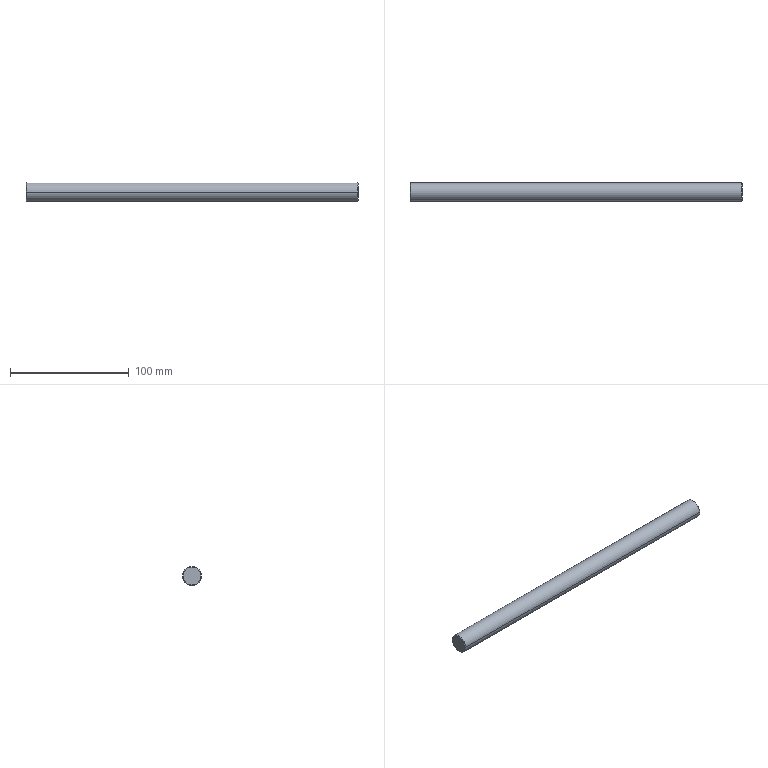Part | STEP file | Guide wheel mechanism revised.sldasm-Part-39 | 1 solid | 12 faces | box 280 x 16 x 16 mm | volume 56107 mm3 | cone 6 | cylinder 4 | plane 2 | commonest cylinder face diameters 4.2 x2 16 x2
STEP:
#1=CARTESIAN_POINT('',(267.6,0.,2.1));
#2=VERTEX_POINT('',#1);
#3=CARTESIAN_POINT('',(267.6,0.,-2.1));
#4=VERTEX_POINT('',#3);
#5=CARTESIAN_POINT('',(267.6,0.,0.));
#6=DIRECTION('',(1.,0.,0.));
#7=DIRECTION('',(0.,0.,-1.));
#8=AXIS2_PLACEMENT_3D('',#5,#6,#7);
#9=CIRCLE('',#8,2.1);
#10=EDGE_CURVE('',#2,#4,#9,.T.);
#11=ORIENTED_EDGE('',*,*,#10,.F.);
#12=CARTESIAN_POINT('',(280.,0.,2.1));
#13=VERTEX_POINT('',#12);
#14=CARTESIAN_POINT('',(280.,0.,2.1));
#15=DIRECTION('',(1.,0.,0.));
#16=VECTOR('',#15,1000.);
#17=LINE('',#14,#16);
#18=EDGE_CURVE('',#2,#13,#17,.T.);
#19=ORIENTED_EDGE('',*,*,#18,.T.);
#20=CARTESIAN_POINT('',(280.,0.,-2.1));
#21=VERTEX_POINT('',#20);
#22=CARTESIAN_POINT('',(280.,0.,0.));
#23=DIRECTION('',(1.,0.,0.));
#24=DIRECTION('',(0.,0.,-1.));
#25=AXIS2_PLACEMENT_3D('',#22,#23,#24);
#26=CIRCLE('',#25,2.1);
#27=EDGE_CURVE('',#13,#21,#26,.T.);
#28=ORIENTED_EDGE('',*,*,#27,.T.);
#29=CARTESIAN_POINT('',(280.,0.,-2.1));
#30=DIRECTION('',(1.,0.,0.));
#31=VECTOR('',#30,1000.);
#32=LINE('',#29,#31);
#33=EDGE_CURVE('',#4,#21,#32,.T.);
#34=ORIENTED_EDGE('',*,*,#33,.F.);
#35=EDGE_LOOP('',(#11,#19,#28,#34));
#36=FACE_OUTER_BOUND('',#35,.T.);
#37=CARTESIAN_POINT('',(280.,0.,0.));
#38=DIRECTION('',(1.,0.,0.));
#39=DIRECTION('',(0.,0.,-1.));
#40=AXIS2_PLACEMENT_3D('',#37,#38,#39);
#41=CYLINDRICAL_SURFACE('',#40,2.1);
#42=ADVANCED_FACE('',(#36),#41,.F.);
#43=CARTESIAN_POINT('',(266.338,0.,0.));
#44=VERTEX_POINT('',#43);
#45=CARTESIAN_POINT('',(267.6,0.,-2.1));
#46=DIRECTION('',(0.515,0.,-0.8572));
#47=VECTOR('',#46,1000.);
#48=LINE('',#45,#47);
#49=EDGE_CURVE('',#44,#4,#48,.T.);
#50=ORIENTED_EDGE('',*,*,#49,.F.);
#51=CARTESIAN_POINT('',(267.6,0.,2.1));
#52=DIRECTION('',(0.515,0.,0.8572));
#53=VECTOR('',#52,1000.);
#54=LINE('',#51,#53);
#55=EDGE_CURVE('',#44,#2,#54,.T.);
#56=ORIENTED_EDGE('',*,*,#55,.T.);
#57=ORIENTED_EDGE('',*,*,#10,.T.);
#58=EDGE_LOOP('',(#50,#56,#57));
#59=FACE_OUTER_BOUND('',#58,.T.);
#60=CARTESIAN_POINT('',(267.6,0.,0.));
#61=DIRECTION('',(1.,0.,0.));
#62=DIRECTION('',(0.,0.,-1.));
#63=AXIS2_PLACEMENT_3D('',#60,#61,#62);
#64=CONICAL_SURFACE('',#63,2.1,1.03);
#65=ADVANCED_FACE('',(#59),#64,.F.);
#66=CARTESIAN_POINT('',(280.,-7.5,0.));
#67=VERTEX_POINT('',#66);
#68=CARTESIAN_POINT('',(280.,7.5,0.));
#69=VERTEX_POINT('',#68);
#70=CARTESIAN_POINT('',(280.,0.,0.));
#71=DIRECTION('',(-1.,0.,0.));
#72=DIRECTION('',(0.,-1.,0.));
#73=AXIS2_PLACEMENT_3D('',#70,#71,#72);
#74=CIRCLE('',#73,7.5);
#75=EDGE_CURVE('',#67,#69,#74,.T.);
#76=ORIENTED_EDGE('',*,*,#75,.T.);
#77=CARTESIAN_POINT('',(279.5,8.,0.));
#78=VERTEX_POINT('',#77);
#79=CARTESIAN_POINT('',(280.,7.5,0.));
#80=DIRECTION('',(-0.7071,0.7071,0.));
#81=VECTOR('',#80,1000.);
#82=LINE('',#79,#81);
#83=EDGE_CURVE('',#69,#78,#82,.T.);
#84=ORIENTED_EDGE('',*,*,#83,.T.);
#85=CARTESIAN_POINT('',(279.5,-8.,0.));
#86=VERTEX_POINT('',#85);
#87=CARTESIAN_POINT('',(279.5,0.,0.));
#88=DIRECTION('',(-1.,0.,0.));
#89=DIRECTION('',(0.,-1.,0.));
#90=AXIS2_PLACEMENT_3D('',#87,#88,#89);
#91=CIRCLE('',#90,8.);
#92=EDGE_CURVE('',#86,#78,#91,.T.);
#93=ORIENTED_EDGE('',*,*,#92,.F.);
#94=CARTESIAN_POINT('',(280.,-7.5,0.));
#95=DIRECTION('',(-0.7071,-0.7071,0.));
#96=VECTOR('',#95,1000.);
#97=LINE('',#94,#96);
#98=EDGE_CURVE('',#67,#86,#97,.T.);
#99=ORIENTED_EDGE('',*,*,#98,.F.);
#100=EDGE_LOOP('',(#76,#84,#93,#99));
#101=FACE_OUTER_BOUND('',#100,.T.);
#102=CARTESIAN_POINT('',(280.,0.,0.));
#103=DIRECTION('',(-1.,0.,0.));
#104=DIRECTION('',(0.,-1.,0.));
#105=AXIS2_PLACEMENT_3D('',#102,#103,#104);
#106=CONICAL_SURFACE('',#105,7.5,0.7854);
#107=ADVANCED_FACE('',(#101),#106,.T.);
#108=ORIENTED_EDGE('',*,*,#92,.T.);
#109=CARTESIAN_POINT('',(0.5,8.,0.));
#110=VERTEX_POINT('',#109);
#111=CARTESIAN_POINT('',(280.,8.,0.));
#112=DIRECTION('',(-1.,0.,0.));
#113=VECTOR('',#112,1000.);
#114=LINE('',#111,#113);
#115=EDGE_CURVE('',#78,#110,#114,.T.);
#116=ORIENTED_EDGE('',*,*,#115,.T.);
#117=CARTESIAN_POINT('',(0.5,-8.,0.));
#118=VERTEX_POINT('',#117);
#119=CARTESIAN_POINT('',(0.5,0.,0.));
#120=DIRECTION('',(-1.,0.,0.));
#121=DIRECTION('',(0.,-1.,0.));
#122=AXIS2_PLACEMENT_3D('',#119,#120,#121);
#123=CIRCLE('',#122,8.);
#124=EDGE_CURVE('',#118,#110,#123,.T.);
#125=ORIENTED_EDGE('',*,*,#124,.F.);
#126=CARTESIAN_POINT('',(280.,-8.,0.));
#127=DIRECTION('',(-1.,0.,0.));
#128=VECTOR('',#127,1000.);
#129=LINE('',#126,#128);
#130=EDGE_CURVE('',#86,#118,#129,.T.);
#131=ORIENTED_EDGE('',*,*,#130,.F.);
#132=EDGE_LOOP('',(#108,#116,#125,#131));
#133=FACE_OUTER_BOUND('',#132,.T.);
#134=CARTESIAN_POINT('',(280.,0.,0.));
#135=DIRECTION('',(-1.,0.,0.));
#136=DIRECTION('',(0.,-1.,0.));
#137=AXIS2_PLACEMENT_3D('',#134,#135,#136);
#138=CYLINDRICAL_SURFACE('',#137,8.);
#139=ADVANCED_FACE('',(#133),#138,.T.);
#140=CARTESIAN_POINT('',(0.,-7.5,0.));
#141=VERTEX_POINT('',#140);
#142=CARTESIAN_POINT('',(0.,7.5,0.));
#143=VERTEX_POINT('',#142);
#144=CARTESIAN_POINT('',(0.,0.,0.));
#145=DIRECTION('',(-1.,0.,0.));
#146=DIRECTION('',(0.,-1.,0.));
#147=AXIS2_PLACEMENT_3D('',#144,#145,#146);
#148=CIRCLE('',#147,7.5);
#149=EDGE_CURVE('',#141,#143,#148,.T.);
#150=ORIENTED_EDGE('',*,*,#149,.F.);
#151=CARTESIAN_POINT('',(0.5,-8.,0.));
#152=DIRECTION('',(0.7071,-0.7071,0.));
#153=VECTOR('',#152,1000.);
#154=LINE('',#151,#153);
#155=EDGE_CURVE('',#141,#118,#154,.T.);
#156=ORIENTED_EDGE('',*,*,#155,.T.);
#157=ORIENTED_EDGE('',*,*,#124,.T.);
#158=CARTESIAN_POINT('',(0.5,8.,0.));
#159=DIRECTION('',(0.7071,0.7071,0.));
#160=VECTOR('',#159,1000.);
#161=LINE('',#158,#160);
#162=EDGE_CURVE('',#143,#110,#161,.T.);
#163=ORIENTED_EDGE('',*,*,#162,.F.);
#164=EDGE_LOOP('',(#150,#156,#157,#163));
#165=FACE_OUTER_BOUND('',#164,.T.);
#166=CARTESIAN_POINT('',(0.5,0.,0.));
#167=DIRECTION('',(1.,0.,0.));
#168=DIRECTION('',(0.,1.,0.));
#169=AXIS2_PLACEMENT_3D('',#166,#167,#168);
#170=CONICAL_SURFACE('',#169,8.,0.7854);
#171=ADVANCED_FACE('',(#165),#170,.T.);
#172=CARTESIAN_POINT('',(0.,0.,0.));
#173=DIRECTION('',(-1.,0.,0.));
#174=DIRECTION('',(0.,-1.,0.));
#175=AXIS2_PLACEMENT_3D('',#172,#173,#174);
#176=CIRCLE('',#175,7.5);
#177=EDGE_CURVE('',#143,#141,#176,.T.);
#178=ORIENTED_EDGE('',*,*,#177,.T.);
#179=ORIENTED_EDGE('',*,*,#149,.T.);
#180=EDGE_LOOP('',(#178,#179));
#181=FACE_OUTER_BOUND('',#180,.T.);
#182=CARTESIAN_POINT('',(0.,0.,0.));
#183=DIRECTION('',(1.,0.,0.));
#184=DIRECTION('',(0.,1.,0.));
#185=AXIS2_PLACEMENT_3D('',#182,#183,#184);
#186=PLANE('',#185);
#187=ADVANCED_FACE('',(#181),#186,.F.);
#188=ORIENTED_EDGE('',*,*,#155,.F.);
#189=ORIENTED_EDGE('',*,*,#177,.F.);
#190=ORIENTED_EDGE('',*,*,#162,.T.);
#191=CARTESIAN_POINT('',(0.5,0.,0.));
#192=DIRECTION('',(-1.,0.,0.));
#193=DIRECTION('',(0.,-1.,0.));
#194=AXIS2_PLACEMENT_3D('',#191,#192,#193);
#195=CIRCLE('',#194,8.);
#196=EDGE_CURVE('',#110,#118,#195,.T.);
#197=ORIENTED_EDGE('',*,*,#196,.T.);
#198=EDGE_LOOP('',(#188,#189,#190,#197));
#199=FACE_OUTER_BOUND('',#198,.T.);
#200=CARTESIAN_POINT('',(0.5,0.,0.));
#201=DIRECTION('',(1.,0.,0.));
#202=DIRECTION('',(0.,1.,0.));
#203=AXIS2_PLACEMENT_3D('',#200,#201,#202);
#204=CONICAL_SURFACE('',#203,8.,0.7854);
#205=ADVANCED_FACE('',(#199),#204,.T.);
#206=ORIENTED_EDGE('',*,*,#115,.F.);
#207=CARTESIAN_POINT('',(279.5,0.,0.));
#208=DIRECTION('',(-1.,0.,0.));
#209=DIRECTION('',(0.,-1.,0.));
#210=AXIS2_PLACEMENT_3D('',#207,#208,#209);
#211=CIRCLE('',#210,8.);
#212=EDGE_CURVE('',#78,#86,#211,.T.);
#213=ORIENTED_EDGE('',*,*,#212,.T.);
#214=ORIENTED_EDGE('',*,*,#130,.T.);
#215=ORIENTED_EDGE('',*,*,#196,.F.);
#216=EDGE_LOOP('',(#206,#213,#214,#215));
#217=FACE_OUTER_BOUND('',#216,.T.);
#218=CARTESIAN_POINT('',(280.,0.,0.));
#219=DIRECTION('',(-1.,0.,0.));
#220=DIRECTION('',(0.,-1.,0.));
#221=AXIS2_PLACEMENT_3D('',#218,#219,#220);
#222=CYLINDRICAL_SURFACE('',#221,8.);
#223=ADVANCED_FACE('',(#217),#222,.T.);
#224=ORIENTED_EDGE('',*,*,#83,.F.);
#225=CARTESIAN_POINT('',(280.,0.,0.));
#226=DIRECTION('',(-1.,0.,0.));
#227=DIRECTION('',(0.,-1.,0.));
#228=AXIS2_PLACEMENT_3D('',#225,#226,#227);
#229=CIRCLE('',#228,7.5);
#230=EDGE_CURVE('',#69,#67,#229,.T.);
#231=ORIENTED_EDGE('',*,*,#230,.T.);
#232=ORIENTED_EDGE('',*,*,#98,.T.);
#233=ORIENTED_EDGE('',*,*,#212,.F.);
#234=EDGE_LOOP('',(#224,#231,#232,#233));
#235=FACE_OUTER_BOUND('',#234,.T.);
#236=CARTESIAN_POINT('',(280.,0.,0.));
#237=DIRECTION('',(-1.,0.,0.));
#238=DIRECTION('',(0.,-1.,0.));
#239=AXIS2_PLACEMENT_3D('',#236,#237,#238);
#240=CONICAL_SURFACE('',#239,7.5,0.7854);
#241=ADVANCED_FACE('',(#235),#240,.T.);
#242=CARTESIAN_POINT('',(280.,0.,0.));
#243=DIRECTION('',(1.,0.,0.));
#244=DIRECTION('',(0.,0.,-1.));
#245=AXIS2_PLACEMENT_3D('',#242,#243,#244);
#246=CIRCLE('',#245,2.1);
#247=EDGE_CURVE('',#21,#13,#246,.T.);
#248=ORIENTED_EDGE('',*,*,#247,.F.);
#249=ORIENTED_EDGE('',*,*,#27,.F.);
#250=EDGE_LOOP('',(#248,#249));
#251=FACE_BOUND('',#250,.T.);
#252=ORIENTED_EDGE('',*,*,#75,.F.);
#253=ORIENTED_EDGE('',*,*,#230,.F.);
#254=EDGE_LOOP('',(#252,#253));
#255=FACE_OUTER_BOUND('',#254,.T.);
#256=CARTESIAN_POINT('',(280.,7.5,0.));
#257=DIRECTION('',(-1.,0.,0.));
#258=DIRECTION('',(0.,-1.,0.));
#259=AXIS2_PLACEMENT_3D('',#256,#257,#258);
#260=PLANE('',#259);
#261=ADVANCED_FACE('',(#251,#255),#260,.F.);
#262=ORIENTED_EDGE('',*,*,#55,.F.);
#263=ORIENTED_EDGE('',*,*,#49,.T.);
#264=CARTESIAN_POINT('',(267.6,0.,0.));
#265=DIRECTION('',(1.,0.,0.));
#266=DIRECTION('',(0.,0.,-1.));
#267=AXIS2_PLACEMENT_3D('',#264,#265,#266);
#268=CIRCLE('',#267,2.1);
#269=EDGE_CURVE('',#4,#2,#268,.T.);
#270=ORIENTED_EDGE('',*,*,#269,.T.);
#271=EDGE_LOOP('',(#262,#263,#270));
#272=FACE_OUTER_BOUND('',#271,.T.);
#273=CARTESIAN_POINT('',(267.6,0.,0.));
#274=DIRECTION('',(1.,0.,0.));
#275=DIRECTION('',(0.,0.,-1.));
#276=AXIS2_PLACEMENT_3D('',#273,#274,#275);
#277=CONICAL_SURFACE('',#276,2.1,1.03);
#278=ADVANCED_FACE('',(#272),#277,.F.);
#279=ORIENTED_EDGE('',*,*,#18,.F.);
#280=ORIENTED_EDGE('',*,*,#269,.F.);
#281=ORIENTED_EDGE('',*,*,#33,.T.);
#282=ORIENTED_EDGE('',*,*,#247,.T.);
#283=EDGE_LOOP('',(#279,#280,#281,#282));
#284=FACE_OUTER_BOUND('',#283,.T.);
#285=CARTESIAN_POINT('',(280.,0.,0.));
#286=DIRECTION('',(1.,0.,0.));
#287=DIRECTION('',(0.,0.,-1.));
#288=AXIS2_PLACEMENT_3D('',#285,#286,#287);
#289=CYLINDRICAL_SURFACE('',#288,2.1);
#290=ADVANCED_FACE('',(#284),#289,.F.);
#291=CLOSED_SHELL('',(#42,#65,#107,#139,#171,#187,#205,#223,#241,#261,#278,#290));
#292=MANIFOLD_SOLID_BREP('',#291);
#293=CARTESIAN_POINT('',(0.,0.,0.));
#294=DIRECTION('',(0.,0.,1.));
#295=DIRECTION('',(1.,0.,0.));
#296=AXIS2_PLACEMENT_3D('',#293,#294,#295);
#297=(LENGTH_UNIT()NAMED_UNIT(*)SI_UNIT(.MILLI.,.METRE.));
#298=UNCERTAINTY_MEASURE_WITH_UNIT(LENGTH_MEASURE(0.00001),#297,'','');
#299=(NAMED_UNIT(*)PLANE_ANGLE_UNIT()SI_UNIT($,.RADIAN.));
#300=(NAMED_UNIT(*)SI_UNIT($,.STERADIAN.)SOLID_ANGLE_UNIT());
#301=(GEOMETRIC_REPRESENTATION_CONTEXT(3)GLOBAL_UNCERTAINTY_ASSIGNED_CONTEXT((#298))GLOBAL_UNIT_ASSIGNED_CONTEXT((#297,#299,#300))REPRESENTATION_CONTEXT('',''));
#302=ADVANCED_BREP_SHAPE_REPRESENTATION('',(#292,#296),#301);